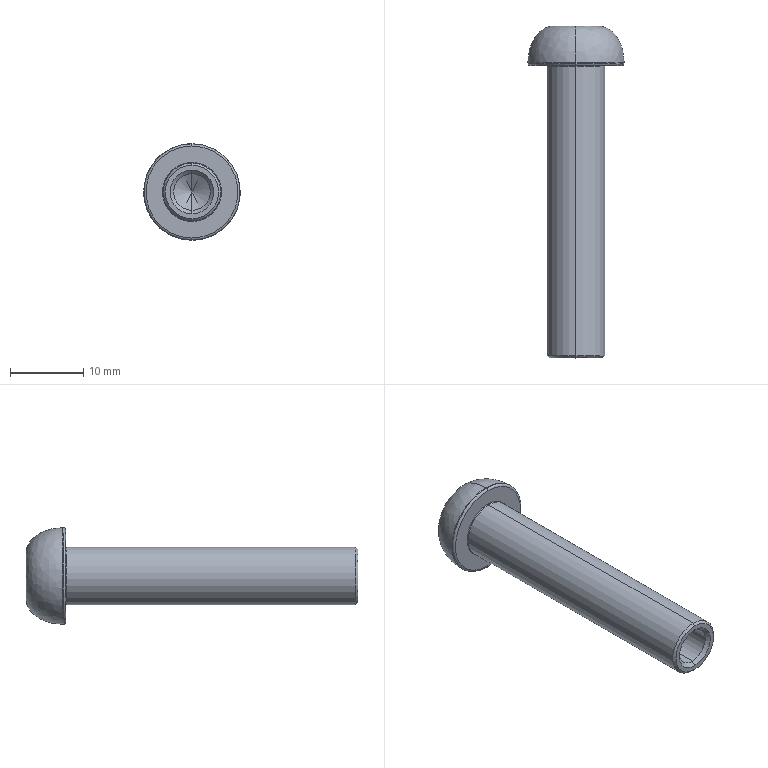Part | SolidWorks | features BaseBody 1 | 1 solid | 38 faces | box 13.2 x 45.4 x 13.2 mm | volume 2174 mm3 | plane 20 | cone 6 | cylinder 6 | torus 4 | spline 2 | commonest cylinder face diameters 5 x2 7.9 x2 13.2 x2
STEP:
#1=CARTESIAN_POINT('',(376.812,-23.5,148.8));
#2=VERTEX_POINT('',#1);
#3=CARTESIAN_POINT('',(376.812,-23.5,153.8));
#4=VERTEX_POINT('',#3);
#5=CARTESIAN_POINT('',(376.812,-23.5,151.3));
#6=DIRECTION('',(0.,1.,0.));
#7=DIRECTION('',(0.,0.,-1.));
#8=AXIS2_PLACEMENT_3D('',#5,#6,#7);
#9=CIRCLE('',#8,2.5);
#10=EDGE_CURVE('',#2,#4,#9,.T.);
#11=ORIENTED_EDGE('',*,*,#10,.T.);
#12=CARTESIAN_POINT('',(376.812,-24.,154.3));
#13=VERTEX_POINT('',#12);
#14=CARTESIAN_POINT('',(376.812,-23.75,154.05));
#15=DIRECTION('',(0.,-0.7071,0.7071));
#16=VECTOR('',#15,1000.);
#17=LINE('',#14,#16);
#18=EDGE_CURVE('',#4,#13,#17,.T.);
#19=ORIENTED_EDGE('',*,*,#18,.T.);
#20=CARTESIAN_POINT('',(376.812,-24.,148.3));
#21=VERTEX_POINT('',#20);
#22=CARTESIAN_POINT('',(376.812,-24.,151.3));
#23=DIRECTION('',(0.,1.,0.));
#24=DIRECTION('',(0.,0.,-1.));
#25=AXIS2_PLACEMENT_3D('',#22,#23,#24);
#26=CIRCLE('',#25,3.);
#27=EDGE_CURVE('',#21,#13,#26,.T.);
#28=ORIENTED_EDGE('',*,*,#27,.F.);
#29=CARTESIAN_POINT('',(376.812,-23.75,148.55));
#30=DIRECTION('',(0.,-0.7071,-0.7071));
#31=VECTOR('',#30,1000.);
#32=LINE('',#29,#31);
#33=EDGE_CURVE('',#2,#21,#32,.T.);
#34=ORIENTED_EDGE('',*,*,#33,.F.);
#35=EDGE_LOOP('',(#11,#19,#28,#34));
#36=FACE_OUTER_BOUND('',#35,.T.);
#37=CARTESIAN_POINT('',(376.812,-23.75,151.3));
#38=DIRECTION('',(0.,-1.,0.));
#39=DIRECTION('',(0.,0.,-1.));
#40=AXIS2_PLACEMENT_3D('',#37,#38,#39);
#41=CONICAL_SURFACE('',#40,2.75,0.7854);
#42=ADVANCED_FACE('',(#36),#41,.F.);
#43=CARTESIAN_POINT('',(376.812,-9.,153.8));
#44=VERTEX_POINT('',#43);
#45=CARTESIAN_POINT('',(376.812,-9.,148.8));
#46=VERTEX_POINT('',#45);
#47=CARTESIAN_POINT('',(376.812,-9.,151.3));
#48=DIRECTION('',(0.,-1.,0.));
#49=DIRECTION('',(0.,0.,1.));
#50=AXIS2_PLACEMENT_3D('',#47,#48,#49);
#51=CIRCLE('',#50,2.5);
#52=EDGE_CURVE('',#44,#46,#51,.T.);
#53=ORIENTED_EDGE('',*,*,#52,.F.);
#54=CARTESIAN_POINT('',(376.812,-9.,153.8));
#55=DIRECTION('',(0.,-1.,0.));
#56=VECTOR('',#55,1000.);
#57=LINE('',#54,#56);
#58=EDGE_CURVE('',#44,#4,#57,.T.);
#59=ORIENTED_EDGE('',*,*,#58,.T.);
#60=ORIENTED_EDGE('',*,*,#10,.F.);
#61=CARTESIAN_POINT('',(376.812,-9.,148.8));
#62=DIRECTION('',(0.,-1.,0.));
#63=VECTOR('',#62,1000.);
#64=LINE('',#61,#63);
#65=EDGE_CURVE('',#46,#2,#64,.T.);
#66=ORIENTED_EDGE('',*,*,#65,.F.);
#67=EDGE_LOOP('',(#53,#59,#60,#66));
#68=FACE_OUTER_BOUND('',#67,.T.);
#69=CARTESIAN_POINT('',(376.812,-9.,151.3));
#70=DIRECTION('',(0.,-1.,0.));
#71=DIRECTION('',(0.,0.,-1.));
#72=AXIS2_PLACEMENT_3D('',#69,#70,#71);
#73=CYLINDRICAL_SURFACE('',#72,2.5);
#74=ADVANCED_FACE('',(#68),#73,.F.);
#75=CARTESIAN_POINT('',(376.812,-7.557,151.3));
#76=VERTEX_POINT('',#75);
#77=CARTESIAN_POINT('',(376.812,-8.293,150.024));
#78=DIRECTION('',(0.,-0.5,-0.866));
#79=VECTOR('',#78,1000.);
#80=LINE('',#77,#79);
#81=EDGE_CURVE('',#76,#46,#80,.T.);
#82=ORIENTED_EDGE('',*,*,#81,.F.);
#83=CARTESIAN_POINT('',(376.812,-8.293,152.576));
#84=DIRECTION('',(0.,-0.5,0.866));
#85=VECTOR('',#84,1000.);
#86=LINE('',#83,#85);
#87=EDGE_CURVE('',#76,#44,#86,.T.);
#88=ORIENTED_EDGE('',*,*,#87,.T.);
#89=ORIENTED_EDGE('',*,*,#52,.T.);
#90=EDGE_LOOP('',(#82,#88,#89));
#91=FACE_OUTER_BOUND('',#90,.T.);
#92=CARTESIAN_POINT('',(376.812,-8.293,151.3));
#93=DIRECTION('',(0.,-1.,0.));
#94=DIRECTION('',(0.,0.,-1.));
#95=AXIS2_PLACEMENT_3D('',#92,#93,#94);
#96=CONICAL_SURFACE('',#95,1.276,1.047);
#97=ADVANCED_FACE('',(#91),#96,.F.);
#98=CARTESIAN_POINT('',(376.812,16.,147.25));
#99=VERTEX_POINT('',#98);
#100=CARTESIAN_POINT('',(376.812,16.,155.35));
#101=VERTEX_POINT('',#100);
#102=CARTESIAN_POINT('',(376.812,16.,151.3));
#103=DIRECTION('',(0.,1.,0.));
#104=DIRECTION('',(0.,0.,-1.));
#105=AXIS2_PLACEMENT_3D('',#102,#103,#104);
#106=CIRCLE('',#105,4.05);
#107=EDGE_CURVE('',#99,#101,#106,.T.);
#108=ORIENTED_EDGE('',*,*,#107,.F.);
#109=CARTESIAN_POINT('',(376.812,15.9,147.35));
#110=VERTEX_POINT('',#109);
#111=CARTESIAN_POINT('',(376.812,15.9,147.25));
#112=DIRECTION('',(1.,0.,0.));
#113=DIRECTION('',(0.,0.,-1.));
#114=AXIS2_PLACEMENT_3D('',#111,#112,#113);
#115=CIRCLE('',#114,0.1);
#116=EDGE_CURVE('',#99,#110,#115,.T.);
#117=ORIENTED_EDGE('',*,*,#116,.T.);
#118=CARTESIAN_POINT('',(376.812,15.9,155.25));
#119=VERTEX_POINT('',#118);
#120=CARTESIAN_POINT('',(376.812,15.9,151.3));
#121=DIRECTION('',(0.,1.,0.));
#122=DIRECTION('',(0.,0.,-1.));
#123=AXIS2_PLACEMENT_3D('',#120,#121,#122);
#124=CIRCLE('',#123,3.95);
#125=EDGE_CURVE('',#110,#119,#124,.T.);
#126=ORIENTED_EDGE('',*,*,#125,.T.);
#127=CARTESIAN_POINT('',(376.812,15.9,155.35));
#128=DIRECTION('',(-1.,0.,0.));
#129=DIRECTION('',(0.,0.,1.));
#130=AXIS2_PLACEMENT_3D('',#127,#128,#129);
#131=CIRCLE('',#130,0.1);
#132=EDGE_CURVE('',#101,#119,#131,.T.);
#133=ORIENTED_EDGE('',*,*,#132,.F.);
#134=EDGE_LOOP('',(#108,#117,#126,#133));
#135=FACE_OUTER_BOUND('',#134,.T.);
#136=CARTESIAN_POINT('',(376.812,15.9,151.3));
#137=DIRECTION('',(0.,1.,0.));
#138=DIRECTION('',(0.,0.,1.));
#139=AXIS2_PLACEMENT_3D('',#136,#137,#138);
#140=TOROIDAL_SURFACE('',#139,4.05,0.1);
#141=ADVANCED_FACE('',(#135),#140,.F.);
#142=CARTESIAN_POINT('',(376.812,16.4,157.9));
#143=VERTEX_POINT('',#142);
#144=CARTESIAN_POINT('',(376.812,16.4,144.7));
#145=VERTEX_POINT('',#144);
#146=CARTESIAN_POINT('',(376.812,16.4,157.9));
#147=CARTESIAN_POINT('',(390.012,16.4,157.9));
#148=CARTESIAN_POINT('',(390.012,16.4,144.7));
#149=CARTESIAN_POINT('',(376.812,16.4,144.7));
#150=(BOUNDED_CURVE()B_SPLINE_CURVE(3,(#146,#147,#148,#149),.UNSPECIFIED.,.F.,.F.)B_SPLINE_CURVE_WITH_KNOTS((4,4),(0.,1.),.UNSPECIFIED.)CURVE()GEOMETRIC_REPRESENTATION_ITEM()RATIONAL_B_SPLINE_CURVE((1.,0.3333,0.3333,1.))REPRESENTATION_ITEM(''));
#151=EDGE_CURVE('',#143,#145,#150,.T.);
#152=ORIENTED_EDGE('',*,*,#151,.F.);
#153=CARTESIAN_POINT('',(376.812,16.3,157.9));
#154=VERTEX_POINT('',#153);
#155=CARTESIAN_POINT('',(376.812,21.4,157.9));
#156=DIRECTION('',(0.,-1.,0.));
#157=VECTOR('',#156,1000.);
#158=LINE('',#155,#157);
#159=EDGE_CURVE('',#143,#154,#158,.T.);
#160=ORIENTED_EDGE('',*,*,#159,.T.);
#161=CARTESIAN_POINT('',(376.812,16.3,144.7));
#162=VERTEX_POINT('',#161);
#163=CARTESIAN_POINT('',(376.812,16.3,151.3));
#164=DIRECTION('',(0.,-1.,0.));
#165=DIRECTION('',(0.,0.,-1.));
#166=AXIS2_PLACEMENT_3D('',#163,#164,#165);
#167=CIRCLE('',#166,6.6);
#168=EDGE_CURVE('',#162,#154,#167,.T.);
#169=ORIENTED_EDGE('',*,*,#168,.F.);
#170=CARTESIAN_POINT('',(376.812,21.4,144.7));
#171=DIRECTION('',(0.,-1.,0.));
#172=VECTOR('',#171,1000.);
#173=LINE('',#170,#172);
#174=EDGE_CURVE('',#145,#162,#173,.T.);
#175=ORIENTED_EDGE('',*,*,#174,.F.);
#176=EDGE_LOOP('',(#152,#160,#169,#175));
#177=FACE_OUTER_BOUND('',#176,.T.);
#178=CARTESIAN_POINT('',(376.812,21.4,151.3));
#179=DIRECTION('',(0.,-1.,0.));
#180=DIRECTION('',(0.,0.,-1.));
#181=AXIS2_PLACEMENT_3D('',#178,#179,#180);
#182=CYLINDRICAL_SURFACE('',#181,6.6);
#183=ADVANCED_FACE('',(#177),#182,.T.);
#184=CARTESIAN_POINT('',(376.812,16.,145.));
#185=VERTEX_POINT('',#184);
#186=CARTESIAN_POINT('',(376.812,16.,157.6));
#187=VERTEX_POINT('',#186);
#188=CARTESIAN_POINT('',(376.812,16.,151.3));
#189=DIRECTION('',(0.,-1.,0.));
#190=DIRECTION('',(0.,0.,1.));
#191=AXIS2_PLACEMENT_3D('',#188,#189,#190);
#192=CIRCLE('',#191,6.3);
#193=EDGE_CURVE('',#185,#187,#192,.T.);
#194=ORIENTED_EDGE('',*,*,#193,.F.);
#195=CARTESIAN_POINT('',(376.812,16.3,145.));
#196=DIRECTION('',(1.,0.,0.));
#197=DIRECTION('',(0.,0.,-1.));
#198=AXIS2_PLACEMENT_3D('',#195,#196,#197);
#199=CIRCLE('',#198,0.3);
#200=EDGE_CURVE('',#185,#162,#199,.T.);
#201=ORIENTED_EDGE('',*,*,#200,.T.);
#202=ORIENTED_EDGE('',*,*,#168,.T.);
#203=CARTESIAN_POINT('',(376.812,16.3,157.6));
#204=DIRECTION('',(-1.,0.,0.));
#205=DIRECTION('',(0.,0.,1.));
#206=AXIS2_PLACEMENT_3D('',#203,#204,#205);
#207=CIRCLE('',#206,0.3);
#208=EDGE_CURVE('',#187,#154,#207,.T.);
#209=ORIENTED_EDGE('',*,*,#208,.F.);
#210=EDGE_LOOP('',(#194,#201,#202,#209));
#211=FACE_OUTER_BOUND('',#210,.T.);
#212=CARTESIAN_POINT('',(376.812,16.3,151.3));
#213=DIRECTION('',(0.,1.,0.));
#214=DIRECTION('',(0.,0.,1.));
#215=AXIS2_PLACEMENT_3D('',#212,#213,#214);
#216=TOROIDAL_SURFACE('',#215,6.3,0.3);
#217=ADVANCED_FACE('',(#211),#216,.T.);
#218=CARTESIAN_POINT('',(376.812,-23.7,147.35));
#219=VERTEX_POINT('',#218);
#220=CARTESIAN_POINT('',(376.812,-23.7,155.25));
#221=VERTEX_POINT('',#220);
#222=CARTESIAN_POINT('',(376.812,-23.7,151.3));
#223=DIRECTION('',(0.,-1.,0.));
#224=DIRECTION('',(0.,0.,-1.));
#225=AXIS2_PLACEMENT_3D('',#222,#223,#224);
#226=CIRCLE('',#225,3.95);
#227=EDGE_CURVE('',#219,#221,#226,.T.);
#228=ORIENTED_EDGE('',*,*,#227,.F.);
#229=CARTESIAN_POINT('',(376.812,-24.,147.35));
#230=DIRECTION('',(0.,1.,0.));
#231=VECTOR('',#230,1000.);
#232=LINE('',#229,#231);
#233=EDGE_CURVE('',#219,#110,#232,.T.);
#234=ORIENTED_EDGE('',*,*,#233,.T.);
#235=CARTESIAN_POINT('',(376.812,15.9,151.3));
#236=DIRECTION('',(0.,1.,0.));
#237=DIRECTION('',(0.,0.,-1.));
#238=AXIS2_PLACEMENT_3D('',#235,#236,#237);
#239=CIRCLE('',#238,3.95);
#240=EDGE_CURVE('',#119,#110,#239,.T.);
#241=ORIENTED_EDGE('',*,*,#240,.F.);
#242=CARTESIAN_POINT('',(376.812,-24.,155.25));
#243=DIRECTION('',(0.,1.,0.));
#244=VECTOR('',#243,1000.);
#245=LINE('',#242,#244);
#246=EDGE_CURVE('',#221,#119,#245,.T.);
#247=ORIENTED_EDGE('',*,*,#246,.F.);
#248=EDGE_LOOP('',(#228,#234,#241,#247));
#249=FACE_OUTER_BOUND('',#248,.T.);
#250=CARTESIAN_POINT('',(376.812,-24.,151.3));
#251=DIRECTION('',(0.,1.,0.));
#252=DIRECTION('',(0.,0.,1.));
#253=AXIS2_PLACEMENT_3D('',#250,#251,#252);
#254=CYLINDRICAL_SURFACE('',#253,3.95);
#255=ADVANCED_FACE('',(#249),#254,.T.);
#256=CARTESIAN_POINT('',(376.812,-24.,147.65));
#257=VERTEX_POINT('',#256);
#258=CARTESIAN_POINT('',(376.812,-24.,154.95));
#259=VERTEX_POINT('',#258);
#260=CARTESIAN_POINT('',(376.812,-24.,151.3));
#261=DIRECTION('',(0.,-1.,0.));
#262=DIRECTION('',(0.,0.,-1.));
#263=AXIS2_PLACEMENT_3D('',#260,#261,#262);
#264=CIRCLE('',#263,3.65);
#265=EDGE_CURVE('',#257,#259,#264,.T.);
#266=ORIENTED_EDGE('',*,*,#265,.F.);
#267=CARTESIAN_POINT('',(376.812,-23.85,147.5));
#268=DIRECTION('',(0.,0.7071,-0.7071));
#269=VECTOR('',#268,1000.);
#270=LINE('',#267,#269);
#271=EDGE_CURVE('',#257,#219,#270,.T.);
#272=ORIENTED_EDGE('',*,*,#271,.T.);
#273=ORIENTED_EDGE('',*,*,#227,.T.);
#274=CARTESIAN_POINT('',(376.812,-23.85,155.1));
#275=DIRECTION('',(0.,0.7071,0.7071));
#276=VECTOR('',#275,1000.);
#277=LINE('',#274,#276);
#278=EDGE_CURVE('',#259,#221,#277,.T.);
#279=ORIENTED_EDGE('',*,*,#278,.F.);
#280=EDGE_LOOP('',(#266,#272,#273,#279));
#281=FACE_OUTER_BOUND('',#280,.T.);
#282=CARTESIAN_POINT('',(376.812,-23.85,151.3));
#283=DIRECTION('',(0.,1.,0.));
#284=DIRECTION('',(0.,0.,1.));
#285=AXIS2_PLACEMENT_3D('',#282,#283,#284);
#286=CONICAL_SURFACE('',#285,3.8,0.7854);
#287=ADVANCED_FACE('',(#281),#286,.T.);
#288=ORIENTED_EDGE('',*,*,#27,.T.);
#289=CARTESIAN_POINT('',(376.812,-24.,151.3));
#290=DIRECTION('',(0.,1.,0.));
#291=DIRECTION('',(0.,0.,-1.));
#292=AXIS2_PLACEMENT_3D('',#289,#290,#291);
#293=CIRCLE('',#292,3.);
#294=EDGE_CURVE('',#13,#21,#293,.T.);
#295=ORIENTED_EDGE('',*,*,#294,.T.);
#296=EDGE_LOOP('',(#288,#295));
#297=FACE_BOUND('',#296,.T.);
#298=CARTESIAN_POINT('',(376.812,-24.,151.3));
#299=DIRECTION('',(0.,-1.,0.));
#300=DIRECTION('',(0.,0.,-1.));
#301=AXIS2_PLACEMENT_3D('',#298,#299,#300);
#302=CIRCLE('',#301,3.65);
#303=EDGE_CURVE('',#259,#257,#302,.T.);
#304=ORIENTED_EDGE('',*,*,#303,.T.);
#305=ORIENTED_EDGE('',*,*,#265,.T.);
#306=EDGE_LOOP('',(#304,#305));
#307=FACE_OUTER_BOUND('',#306,.T.);
#308=CARTESIAN_POINT('',(376.812,-24.,151.3));
#309=DIRECTION('',(0.,-1.,0.));
#310=DIRECTION('',(0.,0.,-1.));
#311=AXIS2_PLACEMENT_3D('',#308,#309,#310);
#312=PLANE('',#311);
#313=ADVANCED_FACE('',(#297,#307),#312,.T.);
#314=ORIENTED_EDGE('',*,*,#271,.F.);
#315=ORIENTED_EDGE('',*,*,#303,.F.);
#316=ORIENTED_EDGE('',*,*,#278,.T.);
#317=CARTESIAN_POINT('',(376.812,-23.7,151.3));
#318=DIRECTION('',(0.,-1.,0.));
#319=DIRECTION('',(0.,0.,-1.));
#320=AXIS2_PLACEMENT_3D('',#317,#318,#319);
#321=CIRCLE('',#320,3.95);
#322=EDGE_CURVE('',#221,#219,#321,.T.);
#323=ORIENTED_EDGE('',*,*,#322,.T.);
#324=EDGE_LOOP('',(#314,#315,#316,#323));
#325=FACE_OUTER_BOUND('',#324,.T.);
#326=CARTESIAN_POINT('',(376.812,-23.85,151.3));
#327=DIRECTION('',(0.,1.,0.));
#328=DIRECTION('',(0.,0.,1.));
#329=AXIS2_PLACEMENT_3D('',#326,#327,#328);
#330=CONICAL_SURFACE('',#329,3.8,0.7854);
#331=ADVANCED_FACE('',(#325),#330,.T.);
#332=ORIENTED_EDGE('',*,*,#233,.F.);
#333=ORIENTED_EDGE('',*,*,#322,.F.);
#334=ORIENTED_EDGE('',*,*,#246,.T.);
#335=ORIENTED_EDGE('',*,*,#125,.F.);
#336=EDGE_LOOP('',(#332,#333,#334,#335));
#337=FACE_OUTER_BOUND('',#336,.T.);
#338=CARTESIAN_POINT('',(376.812,-24.,151.3));
#339=DIRECTION('',(0.,1.,0.));
#340=DIRECTION('',(0.,0.,1.));
#341=AXIS2_PLACEMENT_3D('',#338,#339,#340);
#342=CYLINDRICAL_SURFACE('',#341,3.95);
#343=ADVANCED_FACE('',(#337),#342,.T.);
#344=CARTESIAN_POINT('',(376.812,16.,151.3));
#345=DIRECTION('',(0.,1.,0.));
#346=DIRECTION('',(0.,0.,-1.));
#347=AXIS2_PLACEMENT_3D('',#344,#345,#346);
#348=CIRCLE('',#347,4.05);
#349=EDGE_CURVE('',#101,#99,#348,.T.);
#350=ORIENTED_EDGE('',*,*,#349,.T.);
#351=ORIENTED_EDGE('',*,*,#107,.T.);
#352=EDGE_LOOP('',(#350,#351));
#353=FACE_BOUND('',#352,.T.);
#354=CARTESIAN_POINT('',(376.812,16.,151.3));
#355=DIRECTION('',(0.,-1.,0.));
#356=DIRECTION('',(0.,0.,1.));
#357=AXIS2_PLACEMENT_3D('',#354,#355,#356);
#358=CIRCLE('',#357,6.3);
#359=EDGE_CURVE('',#187,#185,#358,.T.);
#360=ORIENTED_EDGE('',*,*,#359,.T.);
#361=ORIENTED_EDGE('',*,*,#193,.T.);
#362=EDGE_LOOP('',(#360,#361));
#363=FACE_OUTER_BOUND('',#362,.T.);
#364=CARTESIAN_POINT('',(376.812,16.,151.3));
#365=DIRECTION('',(0.,1.,0.));
#366=DIRECTION('',(1.,0.,0.));
#367=AXIS2_PLACEMENT_3D('',#364,#365,#366);
#368=PLANE('',#367);
#369=ADVANCED_FACE('',(#353,#363),#368,.F.);
#370=ORIENTED_EDGE('',*,*,#200,.F.);
#371=ORIENTED_EDGE('',*,*,#359,.F.);
#372=ORIENTED_EDGE('',*,*,#208,.T.);
#373=CARTESIAN_POINT('',(376.812,16.3,151.3));
#374=DIRECTION('',(0.,-1.,0.));
#375=DIRECTION('',(0.,0.,-1.));
#376=AXIS2_PLACEMENT_3D('',#373,#374,#375);
#377=CIRCLE('',#376,6.6);
#378=EDGE_CURVE('',#154,#162,#377,.T.);
#379=ORIENTED_EDGE('',*,*,#378,.T.);
#380=EDGE_LOOP('',(#370,#371,#372,#379));
#381=FACE_OUTER_BOUND('',#380,.T.);
#382=CARTESIAN_POINT('',(376.812,16.3,151.3));
#383=DIRECTION('',(0.,1.,0.));
#384=DIRECTION('',(0.,0.,1.));
#385=AXIS2_PLACEMENT_3D('',#382,#383,#384);
#386=TOROIDAL_SURFACE('',#385,6.3,0.3);
#387=ADVANCED_FACE('',(#381),#386,.T.);
#388=CARTESIAN_POINT('',(376.032,21.4,154.3));
#389=VERTEX_POINT('',#388);
#390=CARTESIAN_POINT('',(376.812,21.4,154.4));
#391=VERTEX_POINT('',#390);
#392=CARTESIAN_POINT('',(376.032,21.4,154.3));
#393=CARTESIAN_POINT('',(376.287,21.4,154.367));
#394=CARTESIAN_POINT('',(376.548,21.4,154.4));
#395=CARTESIAN_POINT('',(376.812,21.4,154.4));
#396=B_SPLINE_CURVE_WITH_KNOTS('',3,(#392,#393,#394,#395),.UNSPECIFIED.,.F.,.F.,(4,4),(0.,1.),.UNSPECIFIED.);
#397=EDGE_CURVE('',#389,#391,#396,.T.);
#398=ORIENTED_EDGE('',*,*,#397,.F.);
#399=CARTESIAN_POINT('',(375.08,21.373,154.3));
#400=VERTEX_POINT('',#399);
#401=CARTESIAN_POINT('',(376.032,21.4,154.3));
#402=CARTESIAN_POINT('',(375.714,21.4,154.3));
#403=CARTESIAN_POINT('',(375.397,21.396,154.3));
#404=CARTESIAN_POINT('',(375.08,21.373,154.3));
#405=B_SPLINE_CURVE_WITH_KNOTS('',3,(#401,#402,#403,#404),.UNSPECIFIED.,.F.,.F.,(4,4),(0.,0.0009518),.UNSPECIFIED.);
#406=EDGE_CURVE('',#389,#400,#405,.T.);
#407=ORIENTED_EDGE('',*,*,#406,.T.);
#408=CARTESIAN_POINT('',(374.605,21.4,153.476));
#409=VERTEX_POINT('',#408);
#410=CARTESIAN_POINT('',(375.08,21.373,154.3));
#411=CARTESIAN_POINT('',(374.922,21.396,154.026));
#412=CARTESIAN_POINT('',(374.763,21.4,153.751));
#413=CARTESIAN_POINT('',(374.605,21.4,153.476));
#414=B_SPLINE_CURVE_WITH_KNOTS('',3,(#410,#411,#412,#413),.UNSPECIFIED.,.F.,.F.,(4,4),(0.,0.0009514),.UNSPECIFIED.);
#415=EDGE_CURVE('',#400,#409,#414,.T.);
#416=ORIENTED_EDGE('',*,*,#415,.T.);
#417=CARTESIAN_POINT('',(373.824,21.4,152.124));
#418=VERTEX_POINT('',#417);
#419=CARTESIAN_POINT('',(374.605,21.4,153.476));
#420=CARTESIAN_POINT('',(374.586,21.4,153.457));
#421=CARTESIAN_POINT('',(374.558,21.4,153.428));
#422=CARTESIAN_POINT('',(374.525,21.4,153.393));
#423=CARTESIAN_POINT('',(374.509,21.4,153.375));
#424=CARTESIAN_POINT('',(374.503,21.4,153.367));
#425=CARTESIAN_POINT('',(374.498,21.4,153.362));
#426=CARTESIAN_POINT('',(374.495,21.4,153.358));
#427=CARTESIAN_POINT('',(374.489,21.4,153.352));
#428=CARTESIAN_POINT('',(374.48,21.4,153.342));
#429=CARTESIAN_POINT('',(374.456,21.4,153.314));
#430=CARTESIAN_POINT('',(374.441,21.4,153.297));
#431=CARTESIAN_POINT('',(374.399,21.4,153.247));
#432=CARTESIAN_POINT('',(374.383,21.4,153.227));
#433=CARTESIAN_POINT('',(374.364,21.4,153.203));
#434=CARTESIAN_POINT('',(374.356,21.4,153.193));
#435=CARTESIAN_POINT('',(374.35,21.4,153.184));
#436=CARTESIAN_POINT('',(374.347,21.4,153.181));
#437=CARTESIAN_POINT('',(374.346,21.4,153.179));
#438=CARTESIAN_POINT('',(374.346,21.4,153.18));
#439=CARTESIAN_POINT('',(374.296,21.4,153.113));
#440=CARTESIAN_POINT('',(374.254,21.4,153.054));
#441=CARTESIAN_POINT('',(374.2,21.4,152.972));
#442=CARTESIAN_POINT('',(374.184,21.4,152.946));
#443=CARTESIAN_POINT('',(374.161,21.4,152.91));
#444=CARTESIAN_POINT('',(374.154,21.4,152.898));
#445=CARTESIAN_POINT('',(374.14,21.4,152.875));
#446=CARTESIAN_POINT('',(374.135,21.4,152.865));
#447=CARTESIAN_POINT('',(374.114,21.4,152.829));
#448=CARTESIAN_POINT('',(374.093,21.4,152.793));
#449=CARTESIAN_POINT('',(374.07,21.4,152.75));
#450=CARTESIAN_POINT('',(374.059,21.4,152.729));
#451=CARTESIAN_POINT('',(374.054,21.4,152.72));
#452=CARTESIAN_POINT('',(374.051,21.4,152.714));
#453=CARTESIAN_POINT('',(374.048,21.4,152.709));
#454=CARTESIAN_POINT('',(374.045,21.4,152.703));
#455=CARTESIAN_POINT('',(374.04,21.4,152.693));
#456=CARTESIAN_POINT('',(374.029,21.4,152.671));
#457=CARTESIAN_POINT('',(374.025,21.4,152.662));
#458=CARTESIAN_POINT('',(374.015,21.4,152.642));
#459=CARTESIAN_POINT('',(374.011,21.4,152.632));
#460=CARTESIAN_POINT('',(373.992,21.4,152.59));
#461=CARTESIAN_POINT('',(373.982,21.4,152.567));
#462=CARTESIAN_POINT('',(373.969,21.4,152.538));
#463=CARTESIAN_POINT('',(373.964,21.4,152.525));
#464=CARTESIAN_POINT('',(373.958,21.4,152.512));
#465=CARTESIAN_POINT('',(373.956,21.4,152.508));
#466=CARTESIAN_POINT('',(373.955,21.4,152.505));
#467=CARTESIAN_POINT('',(373.955,21.4,152.505));
#468=CARTESIAN_POINT('',(373.88,21.4,152.325));
#469=CARTESIAN_POINT('',(373.844,21.4,152.198));
#470=CARTESIAN_POINT('',(373.824,21.4,152.124));
#471=B_SPLINE_CURVE_WITH_KNOTS('',3,(#419,#420,#421,#422,#423,#424,#425,#426,#427,#428,#429,#430,#431,#432,#433,#434,#435,#436,#437,#438,#439,#440,#441,#442,#443,#444,#445,#446,#447,#448,#449,#450,#451,#452,#453,#454,#455,#456,#457,#458,#459,#460,#461,#462,#463,#464,#465,#466,#467,#468,#469,#470),.UNSPECIFIED.,.F.,.F.,(4,1,1,1,2,2,2,2,2,1,1,2,2,2,2,2,2,1,1,1,2,2,2,2,2,2,1,1,2,2,4),(0.,0.0625,0.09375,0.1094,0.1172,0.125,0.1563,0.1875,0.2188,0.2344,0.2422,0.2461,0.25,0.375,0.4375,0.4688,0.5,0.5625,0.5938,0.6094,0.6172,0.625,0.6563,0.6719,0.6875,0.7188,0.7344,0.7422,0.7461,0.75,1.),.UNSPECIFIED.);
#472=EDGE_CURVE('',#409,#418,#471,.T.);
#473=ORIENTED_EDGE('',*,*,#472,.T.);
#474=CARTESIAN_POINT('',(373.348,21.373,151.3));
#475=VERTEX_POINT('',#474);
#476=CARTESIAN_POINT('',(373.824,21.4,152.124));
#477=CARTESIAN_POINT('',(373.665,21.4,151.849));
#478=CARTESIAN_POINT('',(373.507,21.396,151.574));
#479=CARTESIAN_POINT('',(373.348,21.373,151.3));
#480=B_SPLINE_CURVE_WITH_KNOTS('',3,(#476,#477,#478,#479),.UNSPECIFIED.,.F.,.F.,(4,4),(0.,0.000952),.UNSPECIFIED.);
#481=EDGE_CURVE('',#418,#475,#480,.T.);
#482=ORIENTED_EDGE('',*,*,#481,.T.);
#483=CARTESIAN_POINT('',(373.824,21.4,150.476));
#484=VERTEX_POINT('',#483);
#485=CARTESIAN_POINT('',(373.348,21.373,151.3));
#486=CARTESIAN_POINT('',(373.507,21.396,151.026));
#487=CARTESIAN_POINT('',(373.665,21.4,150.751));
#488=CARTESIAN_POINT('',(373.824,21.4,150.476));
#489=B_SPLINE_CURVE_WITH_KNOTS('',3,(#485,#486,#487,#488),.UNSPECIFIED.,.F.,.F.,(4,4),(0.,0.000952),.UNSPECIFIED.);
#490=EDGE_CURVE('',#475,#484,#489,.T.);
#491=ORIENTED_EDGE('',*,*,#490,.T.);
#492=CARTESIAN_POINT('',(374.605,21.4,149.124));
#493=VERTEX_POINT('',#492);
#494=CARTESIAN_POINT('',(373.824,21.4,150.476));
#495=CARTESIAN_POINT('',(373.832,21.4,150.448));
#496=CARTESIAN_POINT('',(373.844,21.4,150.407));
#497=CARTESIAN_POINT('',(373.859,21.4,150.359));
#498=CARTESIAN_POINT('',(373.867,21.4,150.335));
#499=CARTESIAN_POINT('',(373.87,21.4,150.325));
#500=CARTESIAN_POINT('',(373.873,21.4,150.318));
#501=CARTESIAN_POINT('',(373.874,21.4,150.313));
#502=CARTESIAN_POINT('',(373.88,21.4,150.298));
#503=CARTESIAN_POINT('',(373.891,21.4,150.264));
#504=CARTESIAN_POINT('',(373.923,21.4,150.176));
#505=CARTESIAN_POINT('',(373.932,21.4,150.152));
#506=CARTESIAN_POINT('',(373.943,21.4,150.126));
#507=CARTESIAN_POINT('',(373.946,21.4,150.118));
#508=CARTESIAN_POINT('',(373.95,21.4,150.109));
#509=CARTESIAN_POINT('',(373.951,21.4,150.105));
#510=CARTESIAN_POINT('',(373.953,21.4,150.102));
#511=CARTESIAN_POINT('',(373.953,21.4,150.1));
#512=CARTESIAN_POINT('',(373.953,21.4,150.1));
#513=CARTESIAN_POINT('',(373.967,21.4,150.067));
#514=CARTESIAN_POINT('',(373.987,21.4,150.02));
#515=CARTESIAN_POINT('',(374.009,21.4,149.974));
#516=CARTESIAN_POINT('',(374.023,21.4,149.944));
#517=CARTESIAN_POINT('',(374.031,21.4,149.928));
#518=CARTESIAN_POINT('',(374.052,21.4,149.885));
#519=CARTESIAN_POINT('',(374.066,21.4,149.857));
#520=CARTESIAN_POINT('',(374.096,21.4,149.802));
#521=CARTESIAN_POINT('',(374.111,21.4,149.775));
#522=CARTESIAN_POINT('',(374.136,21.4,149.733));
#523=CARTESIAN_POINT('',(374.149,21.4,149.712));
#524=CARTESIAN_POINT('',(374.164,21.4,149.687));
#525=CARTESIAN_POINT('',(374.171,21.4,149.675));
#526=CARTESIAN_POINT('',(374.174,21.4,149.67));
#527=CARTESIAN_POINT('',(374.176,21.4,149.666));
#528=CARTESIAN_POINT('',(374.178,21.4,149.663));
#529=CARTESIAN_POINT('',(374.179,21.4,149.662));
#530=CARTESIAN_POINT('',(374.183,21.4,149.655));
#531=CARTESIAN_POINT('',(374.196,21.4,149.634));
#532=CARTESIAN_POINT('',(374.202,21.4,149.625));
#533=CARTESIAN_POINT('',(374.212,21.4,149.61));
#534=CARTESIAN_POINT('',(374.217,21.4,149.602));
#535=CARTESIAN_POINT('',(374.223,21.4,149.593));
#536=CARTESIAN_POINT('',(374.227,21.4,149.586));
#537=CARTESIAN_POINT('',(374.231,21.4,149.581));
#538=CARTESIAN_POINT('',(374.249,21.4,149.554));
#539=CARTESIAN_POINT('',(374.267,21.4,149.528));
#540=CARTESIAN_POINT('',(374.305,21.4,149.474));
#541=CARTESIAN_POINT('',(374.324,21.4,149.449));
#542=CARTESIAN_POINT('',(374.434,21.4,149.305));
#543=CARTESIAN_POINT('',(374.522,21.4,149.207));
#544=CARTESIAN_POINT('',(374.605,21.4,149.124));
#545=B_SPLINE_CURVE_WITH_KNOTS('',3,(#494,#495,#496,#497,#498,#499,#500,#501,#502,#503,#504,#505,#506,#507,#508,#509,#510,#511,#512,#513,#514,#515,#516,#517,#518,#519,#520,#521,#522,#523,#524,#525,#526,#527,#528,#529,#530,#531,#532,#533,#534,#535,#536,#537,#538,#539,#540,#541,#542,#543,#544),.UNSPECIFIED.,.F.,.F.,(4,1,1,1,2,2,2,2,2,1,2,2,1,2,2,2,2,1,1,1,2,2,2,2,1,2,2,2,2,4),(0.,0.0625,0.09375,0.1094,0.1172,0.125,0.1875,0.2188,0.2344,0.2422,0.2461,0.25,0.3125,0.3438,0.375,0.4375,0.5,0.5312,0.5469,0.5547,0.5586,0.5625,0.5937,0.6094,0.6172,0.6211,0.625,0.6875,0.75,1.),.UNSPECIFIED.);
#546=EDGE_CURVE('',#484,#493,#545,.T.);
#547=ORIENTED_EDGE('',*,*,#546,.T.);
#548=CARTESIAN_POINT('',(375.08,21.373,148.3));
#549=VERTEX_POINT('',#548);
#550=CARTESIAN_POINT('',(374.605,21.4,149.124));
#551=CARTESIAN_POINT('',(374.763,21.4,148.849));
#552=CARTESIAN_POINT('',(374.922,21.396,148.574));
#553=CARTESIAN_POINT('',(375.08,21.373,148.3));
#554=B_SPLINE_CURVE_WITH_KNOTS('',3,(#550,#551,#552,#553),.UNSPECIFIED.,.F.,.F.,(4,4),(0.,0.0009514),.UNSPECIFIED.);
#555=EDGE_CURVE('',#493,#549,#554,.T.);
#556=ORIENTED_EDGE('',*,*,#555,.T.);
#557=CARTESIAN_POINT('',(376.032,21.4,148.3));
#558=VERTEX_POINT('',#557);
#559=CARTESIAN_POINT('',(375.08,21.373,148.3));
#560=CARTESIAN_POINT('',(375.397,21.396,148.3));
#561=CARTESIAN_POINT('',(375.714,21.4,148.3));
#562=CARTESIAN_POINT('',(376.032,21.4,148.3));
#563=B_SPLINE_CURVE_WITH_KNOTS('',3,(#559,#560,#561,#562),.UNSPECIFIED.,.F.,.F.,(4,4),(0.,0.0009518),.UNSPECIFIED.);
#564=EDGE_CURVE('',#549,#558,#563,.T.);
#565=ORIENTED_EDGE('',*,*,#564,.T.);
#566=CARTESIAN_POINT('',(376.812,21.4,148.2));
#567=VERTEX_POINT('',#566);
#568=CARTESIAN_POINT('',(376.812,21.4,148.2));
#569=CARTESIAN_POINT('',(376.548,21.4,148.2));
#570=CARTESIAN_POINT('',(376.287,21.4,148.233));
#571=CARTESIAN_POINT('',(376.032,21.4,148.3));
#572=B_SPLINE_CURVE_WITH_KNOTS('',3,(#568,#569,#570,#571),.UNSPECIFIED.,.F.,.F.,(4,4),(0.,1.),.UNSPECIFIED.);
#573=EDGE_CURVE('',#567,#558,#572,.T.);
#574=ORIENTED_EDGE('',*,*,#573,.F.);
#575=CARTESIAN_POINT('',(376.812,16.4,144.7));
#576=CARTESIAN_POINT('',(376.812,16.981,144.7));
#577=CARTESIAN_POINT('',(376.812,18.257,144.848));
#578=CARTESIAN_POINT('',(376.812,20.059,145.657));
#579=CARTESIAN_POINT('',(376.812,21.195,146.916));
#580=CARTESIAN_POINT('',(376.812,21.4,147.8));
#581=CARTESIAN_POINT('',(376.812,21.4,148.2));
#582=B_SPLINE_CURVE_WITH_KNOTS('',3,(#575,#576,#577,#578,#579,#580,#581),.UNSPECIFIED.,.F.,.F.,(4,1,1,1,4),(0.,0.2463,0.5021,0.7579,1.),.UNSPECIFIED.);
#583=EDGE_CURVE('',#145,#567,#582,.T.);
#584=ORIENTED_EDGE('',*,*,#583,.F.);
#585=CARTESIAN_POINT('',(376.812,16.4,144.7));
#586=CARTESIAN_POINT('',(372.946,16.4,144.7));
#587=CARTESIAN_POINT('',(370.213,16.4,147.434));
#588=CARTESIAN_POINT('',(370.213,16.4,151.3));
#589=CARTESIAN_POINT('',(370.213,16.4,155.166));
#590=CARTESIAN_POINT('',(372.946,16.4,157.9));
#591=CARTESIAN_POINT('',(376.812,16.4,157.9));
#592=(BOUNDED_CURVE()B_SPLINE_CURVE(3,(#585,#586,#587,#588,#589,#590,#591),.UNSPECIFIED.,.F.,.F.)B_SPLINE_CURVE_WITH_KNOTS((4,3,4),(0.,0.5,1.),.UNSPECIFIED.)CURVE()GEOMETRIC_REPRESENTATION_ITEM()RATIONAL_B_SPLINE_CURVE((1.,0.8047,0.8047,1.,0.8047,0.8047,1.))REPRESENTATION_ITEM(''));
#593=EDGE_CURVE('',#145,#143,#592,.T.);
#594=ORIENTED_EDGE('',*,*,#593,.T.);
#595=CARTESIAN_POINT('',(376.812,16.4,157.9));
#596=CARTESIAN_POINT('',(376.812,16.981,157.9));
#597=CARTESIAN_POINT('',(376.812,18.257,157.752));
#598=CARTESIAN_POINT('',(376.812,20.059,156.943));
#599=CARTESIAN_POINT('',(376.812,21.195,155.684));
#600=CARTESIAN_POINT('',(376.812,21.4,154.8));
#601=CARTESIAN_POINT('',(376.812,21.4,154.4));
#602=(BOUNDED_CURVE()B_SPLINE_CURVE(3,(#595,#596,#597,#598,#599,#600,#601),.UNSPECIFIED.,.F.,.F.)B_SPLINE_CURVE_WITH_KNOTS((4,1,1,1,4),(0.,0.2463,0.5021,0.7579,1.),.UNSPECIFIED.)CURVE()GEOMETRIC_REPRESENTATION_ITEM()RATIONAL_B_SPLINE_CURVE((1.,1.,1.,1.,1.,1.,1.))REPRESENTATION_ITEM(''));
#603=EDGE_CURVE('',#143,#391,#602,.T.);
#604=ORIENTED_EDGE('',*,*,#603,.T.);
#605=EDGE_LOOP('',(#398,#407,#416,#473,#482,#491,#547,#556,#565,#574,#584,#594,#604));
#606=FACE_OUTER_BOUND('',#605,.T.);
#607=CARTESIAN_POINT('',(376.812,21.4,154.369));
#608=CARTESIAN_POINT('',(375.014,21.4,154.369));
#609=CARTESIAN_POINT('',(373.743,21.4,153.098));
#610=CARTESIAN_POINT('',(373.743,21.4,151.3));
#611=CARTESIAN_POINT('',(373.743,21.4,149.502));
#612=CARTESIAN_POINT('',(375.014,21.4,148.231));
#613=CARTESIAN_POINT('',(376.812,21.4,148.231));
#614=CARTESIAN_POINT('',(376.812,21.405,154.778));
#615=CARTESIAN_POINT('',(374.775,21.405,154.778));
#616=CARTESIAN_POINT('',(373.335,21.405,153.337));
#617=CARTESIAN_POINT('',(373.335,21.405,151.3));
#618=CARTESIAN_POINT('',(373.335,21.405,149.263));
#619=CARTESIAN_POINT('',(374.775,21.405,147.822));
#620=CARTESIAN_POINT('',(376.812,21.405,147.822));
#621=CARTESIAN_POINT('',(376.812,21.204,155.674));
#622=CARTESIAN_POINT('',(374.25,21.204,155.674));
#623=CARTESIAN_POINT('',(372.438,21.204,153.862));
#624=CARTESIAN_POINT('',(372.438,21.204,151.3));
#625=CARTESIAN_POINT('',(372.438,21.204,148.738));
#626=CARTESIAN_POINT('',(374.25,21.204,146.926));
#627=CARTESIAN_POINT('',(376.812,21.204,146.926));
#628=CARTESIAN_POINT('',(376.812,20.059,156.943));
#629=CARTESIAN_POINT('',(373.507,20.059,156.943));
#630=CARTESIAN_POINT('',(371.169,20.059,154.606));
#631=CARTESIAN_POINT('',(371.169,20.059,151.3));
#632=CARTESIAN_POINT('',(371.169,20.059,147.994));
#633=CARTESIAN_POINT('',(373.507,20.059,145.657));
#634=CARTESIAN_POINT('',(376.812,20.059,145.657));
#635=CARTESIAN_POINT('',(376.812,18.257,157.752));
#636=CARTESIAN_POINT('',(373.033,18.257,157.752));
#637=CARTESIAN_POINT('',(370.36,18.257,155.08));
#638=CARTESIAN_POINT('',(370.36,18.257,151.3));
#639=CARTESIAN_POINT('',(370.36,18.257,147.52));
#640=CARTESIAN_POINT('',(373.033,18.257,144.848));
#641=CARTESIAN_POINT('',(376.812,18.257,144.848));
#642=CARTESIAN_POINT('',(376.812,16.981,157.9));
#643=CARTESIAN_POINT('',(372.946,16.981,157.9));
#644=CARTESIAN_POINT('',(370.213,16.981,155.166));
#645=CARTESIAN_POINT('',(370.213,16.981,151.3));
#646=CARTESIAN_POINT('',(370.213,16.981,147.434));
#647=CARTESIAN_POINT('',(372.946,16.981,144.7));
#648=CARTESIAN_POINT('',(376.812,16.981,144.7));
#649=CARTESIAN_POINT('',(376.812,16.4,157.9));
#650=CARTESIAN_POINT('',(372.946,16.4,157.9));
#651=CARTESIAN_POINT('',(370.213,16.4,155.166));
#652=CARTESIAN_POINT('',(370.213,16.4,151.3));
#653=CARTESIAN_POINT('',(370.213,16.4,147.434));
#654=CARTESIAN_POINT('',(372.946,16.4,144.7));
#655=CARTESIAN_POINT('',(376.812,16.4,144.7));
#656=(BOUNDED_SURFACE()B_SPLINE_SURFACE(3,3,((#607,#608,#609,#610,#611,#612,#613),(#614,#615,#616,#617,#618,#619,#620),(#621,#622,#623,#624,#625,#626,#627),(#628,#629,#630,#631,#632,#633,#634),(#635,#636,#637,#638,#639,#640,#641),(#642,#643,#644,#645,#646,#647,#648),(#649,#650,#651,#652,#653,#654,#655)),.UNSPECIFIED.,.F.,.F.,.F.)B_SPLINE_SURFACE_WITH_KNOTS((4,1,1,1,4),(4,3,4),(0.007322,0.25,0.5,0.75,0.9907),(0.,0.5,1.),.UNSPECIFIED.)GEOMETRIC_REPRESENTATION_ITEM()RATIONAL_B_SPLINE_SURFACE(((1.,0.8047,0.8047,1.,0.8047,0.8047,1.),(1.,0.8047,0.8047,1.,0.8047,0.8047,1.),(1.,0.8047,0.8047,1.,0.8047,0.8047,1.),(1.,0.8047,0.8047,1.,0.8047,0.8047,1.),(1.,0.8047,0.8047,1.,0.8047,0.8047,1.),(1.,0.8047,0.8047,1.,0.8047,0.8047,1.),(1.,0.8047,0.8047,1.,0.8047,0.8047,1.)))REPRESENTATION_ITEM('')SURFACE());
#657=ADVANCED_FACE('',(#606),#656,.F.);
#658=ORIENTED_EDGE('',*,*,#603,.F.);
#659=ORIENTED_EDGE('',*,*,#151,.T.);
#660=ORIENTED_EDGE('',*,*,#583,.T.);
#661=CARTESIAN_POINT('',(377.593,21.4,148.3));
#662=VERTEX_POINT('',#661);
#663=CARTESIAN_POINT('',(377.593,21.4,148.3));
#664=CARTESIAN_POINT('',(377.337,21.4,148.233));
#665=CARTESIAN_POINT('',(377.077,21.4,148.2));
#666=CARTESIAN_POINT('',(376.812,21.4,148.2));
#667=B_SPLINE_CURVE_WITH_KNOTS('',3,(#663,#664,#665,#666),.UNSPECIFIED.,.F.,.F.,(4,4),(0.,1.),.UNSPECIFIED.);
#668=EDGE_CURVE('',#662,#567,#667,.T.);
#669=ORIENTED_EDGE('',*,*,#668,.F.);
#670=CARTESIAN_POINT('',(378.544,21.373,148.3));
#671=VERTEX_POINT('',#670);
#672=CARTESIAN_POINT('',(377.593,21.4,148.3));
#673=CARTESIAN_POINT('',(377.91,21.4,148.3));
#674=CARTESIAN_POINT('',(378.228,21.396,148.3));
#675=CARTESIAN_POINT('',(378.544,21.373,148.3));
#676=B_SPLINE_CURVE_WITH_KNOTS('',3,(#672,#673,#674,#675),.UNSPECIFIED.,.F.,.F.,(4,4),(0.,0.0009518),.UNSPECIFIED.);
#677=EDGE_CURVE('',#662,#671,#676,.T.);
#678=ORIENTED_EDGE('',*,*,#677,.T.);
#679=CARTESIAN_POINT('',(379.02,21.4,149.124));
#680=VERTEX_POINT('',#679);
#681=CARTESIAN_POINT('',(378.544,21.373,148.3));
#682=CARTESIAN_POINT('',(378.703,21.396,148.574));
#683=CARTESIAN_POINT('',(378.861,21.4,148.849));
#684=CARTESIAN_POINT('',(379.02,21.4,149.124));
#685=B_SPLINE_CURVE_WITH_KNOTS('',3,(#681,#682,#683,#684),.UNSPECIFIED.,.F.,.F.,(4,4),(0.,0.0009514),.UNSPECIFIED.);
#686=EDGE_CURVE('',#671,#680,#685,.T.);
#687=ORIENTED_EDGE('',*,*,#686,.T.);
#688=CARTESIAN_POINT('',(379.801,21.4,150.476));
#689=VERTEX_POINT('',#688);
#690=CARTESIAN_POINT('',(379.02,21.4,149.124));
#691=CARTESIAN_POINT('',(379.039,21.4,149.143));
#692=CARTESIAN_POINT('',(379.067,21.4,149.172));
#693=CARTESIAN_POINT('',(379.099,21.4,149.207));
#694=CARTESIAN_POINT('',(379.115,21.4,149.225));
#695=CARTESIAN_POINT('',(379.122,21.4,149.233));
#696=CARTESIAN_POINT('',(379.127,21.4,149.238));
#697=CARTESIAN_POINT('',(379.13,21.4,149.242));
#698=CARTESIAN_POINT('',(379.136,21.4,149.248));
#699=CARTESIAN_POINT('',(379.144,21.4,149.258));
#700=CARTESIAN_POINT('',(379.169,21.4,149.286));
#701=CARTESIAN_POINT('',(379.184,21.4,149.303));
#702=CARTESIAN_POINT('',(379.225,21.4,149.353));
#703=CARTESIAN_POINT('',(379.242,21.4,149.374));
#704=CARTESIAN_POINT('',(379.261,21.4,149.397));
#705=CARTESIAN_POINT('',(379.268,21.4,149.407));
#706=CARTESIAN_POINT('',(379.275,21.4,149.416));
#707=CARTESIAN_POINT('',(379.277,21.4,149.419));
#708=CARTESIAN_POINT('',(379.279,21.4,149.421));
#709=CARTESIAN_POINT('',(379.278,21.4,149.42));
#710=CARTESIAN_POINT('',(379.329,21.4,149.487));
#711=CARTESIAN_POINT('',(379.371,21.4,149.547));
#712=CARTESIAN_POINT('',(379.425,21.4,149.629));
#713=CARTESIAN_POINT('',(379.441,21.4,149.655));
#714=CARTESIAN_POINT('',(379.464,21.4,149.691));
#715=CARTESIAN_POINT('',(379.471,21.4,149.703));
#716=CARTESIAN_POINT('',(379.484,21.4,149.725));
#717=CARTESIAN_POINT('',(379.49,21.4,149.735));
#718=CARTESIAN_POINT('',(379.511,21.4,149.771));
#719=CARTESIAN_POINT('',(379.531,21.4,149.807));
#720=CARTESIAN_POINT('',(379.554,21.4,149.85));
#721=CARTESIAN_POINT('',(379.566,21.4,149.871));
#722=CARTESIAN_POINT('',(379.571,21.4,149.88));
#723=CARTESIAN_POINT('',(379.574,21.4,149.886));
#724=CARTESIAN_POINT('',(379.576,21.4,149.891));
#725=CARTESIAN_POINT('',(379.58,21.4,149.897));
#726=CARTESIAN_POINT('',(379.585,21.4,149.907));
#727=CARTESIAN_POINT('',(379.596,21.4,149.929));
#728=CARTESIAN_POINT('',(379.6,21.4,149.938));
#729=CARTESIAN_POINT('',(379.609,21.4,149.958));
#730=CARTESIAN_POINT('',(379.614,21.4,149.968));
#731=CARTESIAN_POINT('',(379.633,21.4,150.01));
#732=CARTESIAN_POINT('',(379.643,21.4,150.034));
#733=CARTESIAN_POINT('',(379.656,21.4,150.063));
#734=CARTESIAN_POINT('',(379.661,21.4,150.076));
#735=CARTESIAN_POINT('',(379.666,21.4,150.088));
#736=CARTESIAN_POINT('',(379.668,21.4,150.092));
#737=CARTESIAN_POINT('',(379.669,21.4,150.095));
#738=CARTESIAN_POINT('',(379.669,21.4,150.095));
#739=CARTESIAN_POINT('',(379.744,21.4,150.274));
#740=CARTESIAN_POINT('',(379.781,21.4,150.404));
#741=CARTESIAN_POINT('',(379.801,21.4,150.476));
#742=B_SPLINE_CURVE_WITH_KNOTS('',3,(#690,#691,#692,#693,#694,#695,#696,#697,#698,#699,#700,#701,#702,#703,#704,#705,#706,#707,#708,#709,#710,#711,#712,#713,#714,#715,#716,#717,#718,#719,#720,#721,#722,#723,#724,#725,#726,#727,#728,#729,#730,#731,#732,#733,#734,#735,#736,#737,#738,#739,#740,#741),.UNSPECIFIED.,.F.,.F.,(4,1,1,1,2,2,2,2,2,1,1,2,2,2,2,2,2,1,1,1,2,2,2,2,2,2,1,1,2,2,4),(0.,0.0625,0.09375,0.1094,0.1172,0.125,0.1563,0.1875,0.2188,0.2344,0.2422,0.2461,0.25,0.375,0.4375,0.4688,0.5,0.5625,0.5938,0.6094,0.6172,0.625,0.6563,0.6719,0.6875,0.7188,0.7344,0.7422,0.7461,0.75,1.),.UNSPECIFIED.);
#743=EDGE_CURVE('',#680,#689,#742,.T.);
#744=ORIENTED_EDGE('',*,*,#743,.T.);
#745=CARTESIAN_POINT('',(380.276,21.373,151.3));
#746=VERTEX_POINT('',#745);
#747=CARTESIAN_POINT('',(379.801,21.4,150.476));
#748=CARTESIAN_POINT('',(379.959,21.4,150.751));
#749=CARTESIAN_POINT('',(380.118,21.396,151.026));
#750=CARTESIAN_POINT('',(380.276,21.373,151.3));
#751=B_SPLINE_CURVE_WITH_KNOTS('',3,(#747,#748,#749,#750),.UNSPECIFIED.,.F.,.F.,(4,4),(0.,0.000952),.UNSPECIFIED.);
#752=EDGE_CURVE('',#689,#746,#751,.T.);
#753=ORIENTED_EDGE('',*,*,#752,.T.);
#754=CARTESIAN_POINT('',(379.801,21.4,152.124));
#755=VERTEX_POINT('',#754);
#756=CARTESIAN_POINT('',(380.276,21.373,151.3));
#757=CARTESIAN_POINT('',(380.118,21.396,151.574));
#758=CARTESIAN_POINT('',(379.959,21.4,151.849));
#759=CARTESIAN_POINT('',(379.801,21.4,152.124));
#760=B_SPLINE_CURVE_WITH_KNOTS('',3,(#756,#757,#758,#759),.UNSPECIFIED.,.F.,.F.,(4,4),(0.,0.000952),.UNSPECIFIED.);
#761=EDGE_CURVE('',#746,#755,#760,.T.);
#762=ORIENTED_EDGE('',*,*,#761,.T.);
#763=CARTESIAN_POINT('',(379.02,21.4,153.476));
#764=VERTEX_POINT('',#763);
#765=CARTESIAN_POINT('',(379.801,21.4,152.124));
#766=CARTESIAN_POINT('',(379.793,21.4,152.152));
#767=CARTESIAN_POINT('',(379.781,21.4,152.193));
#768=CARTESIAN_POINT('',(379.766,21.4,152.241));
#769=CARTESIAN_POINT('',(379.758,21.4,152.265));
#770=CARTESIAN_POINT('',(379.754,21.4,152.275));
#771=CARTESIAN_POINT('',(379.752,21.4,152.282));
#772=CARTESIAN_POINT('',(379.75,21.4,152.287));
#773=CARTESIAN_POINT('',(379.745,21.4,152.302));
#774=CARTESIAN_POINT('',(379.734,21.4,152.336));
#775=CARTESIAN_POINT('',(379.702,21.4,152.424));
#776=CARTESIAN_POINT('',(379.693,21.4,152.447));
#777=CARTESIAN_POINT('',(379.682,21.4,152.474));
#778=CARTESIAN_POINT('',(379.677,21.4,152.485));
#779=CARTESIAN_POINT('',(379.674,21.4,152.495));
#780=CARTESIAN_POINT('',(379.672,21.4,152.498));
#781=CARTESIAN_POINT('',(379.671,21.4,152.5));
#782=CARTESIAN_POINT('',(379.671,21.4,152.5));
#783=CARTESIAN_POINT('',(379.658,21.4,152.533));
#784=CARTESIAN_POINT('',(379.637,21.4,152.58));
#785=CARTESIAN_POINT('',(379.616,21.4,152.626));
#786=CARTESIAN_POINT('',(379.602,21.4,152.656));
#787=CARTESIAN_POINT('',(379.594,21.4,152.672));
#788=CARTESIAN_POINT('',(379.573,21.4,152.715));
#789=CARTESIAN_POINT('',(379.559,21.4,152.743));
#790=CARTESIAN_POINT('',(379.529,21.4,152.798));
#791=CARTESIAN_POINT('',(379.514,21.4,152.825));
#792=CARTESIAN_POINT('',(379.489,21.4,152.867));
#793=CARTESIAN_POINT('',(379.476,21.4,152.888));
#794=CARTESIAN_POINT('',(379.461,21.4,152.913));
#795=CARTESIAN_POINT('',(379.454,21.4,152.925));
#796=CARTESIAN_POINT('',(379.451,21.4,152.93));
#797=CARTESIAN_POINT('',(379.448,21.4,152.934));
#798=CARTESIAN_POINT('',(379.446,21.4,152.937));
#799=CARTESIAN_POINT('',(379.446,21.4,152.938));
#800=CARTESIAN_POINT('',(379.441,21.4,152.945));
#801=CARTESIAN_POINT('',(379.428,21.4,152.966));
#802=CARTESIAN_POINT('',(379.423,21.4,152.975));
#803=CARTESIAN_POINT('',(379.413,21.4,152.99));
#804=CARTESIAN_POINT('',(379.407,21.4,152.998));
#805=CARTESIAN_POINT('',(379.401,21.4,153.007));
#806=CARTESIAN_POINT('',(379.397,21.4,153.014));
#807=CARTESIAN_POINT('',(379.394,21.4,153.019));
#808=CARTESIAN_POINT('',(379.376,21.4,153.046));
#809=CARTESIAN_POINT('',(379.358,21.4,153.072));
#810=CARTESIAN_POINT('',(379.319,21.4,153.126));
#811=CARTESIAN_POINT('',(379.301,21.4,153.151));
#812=CARTESIAN_POINT('',(379.19,21.4,153.296));
#813=CARTESIAN_POINT('',(379.102,21.4,153.394));
#814=CARTESIAN_POINT('',(379.02,21.4,153.476));
#815=B_SPLINE_CURVE_WITH_KNOTS('',3,(#765,#766,#767,#768,#769,#770,#771,#772,#773,#774,#775,#776,#777,#778,#779,#780,#781,#782,#783,#784,#785,#786,#787,#788,#789,#790,#791,#792,#793,#794,#795,#796,#797,#798,#799,#800,#801,#802,#803,#804,#805,#806,#807,#808,#809,#810,#811,#812,#813,#814),.UNSPECIFIED.,.F.,.F.,(4,1,1,1,2,2,2,2,1,1,2,2,1,2,2,2,2,1,1,1,2,2,2,2,1,2,2,2,2,4),(0.,0.0625,0.09375,0.1094,0.1172,0.125,0.1875,0.2188,0.2344,0.2422,0.2461,0.25,0.3125,0.3438,0.375,0.4375,0.5,0.5313,0.5469,0.5547,0.5586,0.5625,0.5938,0.6094,0.6172,0.6211,0.625,0.6875,0.75,1.),.UNSPECIFIED.);
#816=EDGE_CURVE('',#755,#764,#815,.T.);
#817=ORIENTED_EDGE('',*,*,#816,.T.);
#818=CARTESIAN_POINT('',(378.544,21.373,154.3));
#819=VERTEX_POINT('',#818);
#820=CARTESIAN_POINT('',(379.02,21.4,153.476));
#821=CARTESIAN_POINT('',(378.861,21.4,153.751));
#822=CARTESIAN_POINT('',(378.703,21.396,154.026));
#823=CARTESIAN_POINT('',(378.544,21.373,154.3));
#824=B_SPLINE_CURVE_WITH_KNOTS('',3,(#820,#821,#822,#823),.UNSPECIFIED.,.F.,.F.,(4,4),(0.,0.0009514),.UNSPECIFIED.);
#825=EDGE_CURVE('',#764,#819,#824,.T.);
#826=ORIENTED_EDGE('',*,*,#825,.T.);
#827=CARTESIAN_POINT('',(377.593,21.4,154.3));
#828=VERTEX_POINT('',#827);
#829=CARTESIAN_POINT('',(378.544,21.373,154.3));
#830=CARTESIAN_POINT('',(378.228,21.396,154.3));
#831=CARTESIAN_POINT('',(377.91,21.4,154.3));
#832=CARTESIAN_POINT('',(377.593,21.4,154.3));
#833=B_SPLINE_CURVE_WITH_KNOTS('',3,(#829,#830,#831,#832),.UNSPECIFIED.,.F.,.F.,(4,4),(0.,0.0009518),.UNSPECIFIED.);
#834=EDGE_CURVE('',#819,#828,#833,.T.);
#835=ORIENTED_EDGE('',*,*,#834,.T.);
#836=CARTESIAN_POINT('',(376.812,21.4,154.4));
#837=CARTESIAN_POINT('',(377.077,21.4,154.4));
#838=CARTESIAN_POINT('',(377.337,21.4,154.367));
#839=CARTESIAN_POINT('',(377.593,21.4,154.3));
#840=B_SPLINE_CURVE_WITH_KNOTS('',3,(#836,#837,#838,#839),.UNSPECIFIED.,.F.,.F.,(4,4),(0.,1.),.UNSPECIFIED.);
#841=EDGE_CURVE('',#391,#828,#840,.T.);
#842=ORIENTED_EDGE('',*,*,#841,.F.);
#843=EDGE_LOOP('',(#658,#659,#660,#669,#678,#687,#744,#753,#762,#817,#826,#835,#842));
#844=FACE_OUTER_BOUND('',#843,.T.);
#845=CARTESIAN_POINT('',(376.812,21.4,148.231));
#846=CARTESIAN_POINT('',(382.951,21.4,148.231));
#847=CARTESIAN_POINT('',(382.951,21.4,154.369));
#848=CARTESIAN_POINT('',(376.812,21.4,154.369));
#849=CARTESIAN_POINT('',(376.812,21.405,147.822));
#850=CARTESIAN_POINT('',(383.768,21.405,147.822));
#851=CARTESIAN_POINT('',(383.768,21.405,154.778));
#852=CARTESIAN_POINT('',(376.812,21.405,154.778));
#853=CARTESIAN_POINT('',(376.812,21.204,146.926));
#854=CARTESIAN_POINT('',(385.56,21.204,146.926));
#855=CARTESIAN_POINT('',(385.56,21.204,155.674));
#856=CARTESIAN_POINT('',(376.812,21.204,155.674));
#857=CARTESIAN_POINT('',(376.812,20.059,145.657));
#858=CARTESIAN_POINT('',(388.099,20.059,145.657));
#859=CARTESIAN_POINT('',(388.099,20.059,156.943));
#860=CARTESIAN_POINT('',(376.812,20.059,156.943));
#861=CARTESIAN_POINT('',(376.812,18.257,144.848));
#862=CARTESIAN_POINT('',(389.717,18.257,144.848));
#863=CARTESIAN_POINT('',(389.717,18.257,157.752));
#864=CARTESIAN_POINT('',(376.812,18.257,157.752));
#865=CARTESIAN_POINT('',(376.812,16.981,144.7));
#866=CARTESIAN_POINT('',(390.012,16.981,144.7));
#867=CARTESIAN_POINT('',(390.012,16.981,157.9));
#868=CARTESIAN_POINT('',(376.812,16.981,157.9));
#869=CARTESIAN_POINT('',(376.812,16.4,144.7));
#870=CARTESIAN_POINT('',(390.012,16.4,144.7));
#871=CARTESIAN_POINT('',(390.012,16.4,157.9));
#872=CARTESIAN_POINT('',(376.812,16.4,157.9));
#873=(BOUNDED_SURFACE()B_SPLINE_SURFACE(3,3,((#845,#846,#847,#848),(#849,#850,#851,#852),(#853,#854,#855,#856),(#857,#858,#859,#860),(#861,#862,#863,#864),(#865,#866,#867,#868),(#869,#870,#871,#872)),.UNSPECIFIED.,.F.,.F.,.T.)B_SPLINE_SURFACE_WITH_KNOTS((4,1,1,1,4),(4,4),(0.007322,0.25,0.5,0.75,0.9907),(0.,1.),.UNSPECIFIED.)GEOMETRIC_REPRESENTATION_ITEM()RATIONAL_B_SPLINE_SURFACE(((1.,0.3333,0.3333,1.),(1.,0.3333,0.3333,1.),(1.,0.3333,0.3333,1.),(1.,0.3333,0.3333,1.),(1.,0.3333,0.3333,1.),(1.,0.3333,0.3333,1.),(1.,0.3333,0.3333,1.)))REPRESENTATION_ITEM('')SURFACE());
#874=ADVANCED_FACE('',(#844),#873,.F.);
#875=ORIENTED_EDGE('',*,*,#397,.T.);
#876=ORIENTED_EDGE('',*,*,#841,.T.);
#877=CARTESIAN_POINT('',(377.593,21.4,154.3));
#878=DIRECTION('',(-1.,0.,0.));
#879=VECTOR('',#878,1000.);
#880=LINE('',#877,#879);
#881=EDGE_CURVE('',#828,#389,#880,.T.);
#882=ORIENTED_EDGE('',*,*,#881,.T.);
#883=EDGE_LOOP('',(#875,#876,#882));
#884=FACE_OUTER_BOUND('',#883,.T.);
#885=CARTESIAN_POINT('',(376.812,21.4,151.3));
#886=DIRECTION('',(0.,1.,0.));
#887=DIRECTION('',(1.,0.,0.));
#888=AXIS2_PLACEMENT_3D('',#885,#886,#887);
#889=PLANE('',#888);
#890=ADVANCED_FACE('',(#884),#889,.T.);
#891=ORIENTED_EDGE('',*,*,#406,.F.);
#892=ORIENTED_EDGE('',*,*,#881,.F.);
#893=ORIENTED_EDGE('',*,*,#834,.F.);
#894=CARTESIAN_POINT('',(378.544,19.4,154.3));
#895=VERTEX_POINT('',#894);
#896=CARTESIAN_POINT('',(378.544,19.4,154.3));
#897=DIRECTION('',(0.,-1.,0.));
#898=VECTOR('',#897,1000.);
#899=LINE('',#896,#898);
#900=EDGE_CURVE('',#819,#895,#899,.T.);
#901=ORIENTED_EDGE('',*,*,#900,.T.);
#902=CARTESIAN_POINT('',(375.08,19.4,154.3));
#903=VERTEX_POINT('',#902);
#904=CARTESIAN_POINT('',(378.544,19.4,154.3));
#905=DIRECTION('',(-1.,0.,0.));
#906=VECTOR('',#905,1000.);
#907=LINE('',#904,#906);
#908=EDGE_CURVE('',#895,#903,#907,.T.);
#909=ORIENTED_EDGE('',*,*,#908,.T.);
#910=CARTESIAN_POINT('',(375.08,19.4,154.3));
#911=DIRECTION('',(0.,-1.,0.));
#912=VECTOR('',#911,1000.);
#913=LINE('',#910,#912);
#914=EDGE_CURVE('',#400,#903,#913,.T.);
#915=ORIENTED_EDGE('',*,*,#914,.F.);
#916=EDGE_LOOP('',(#891,#892,#893,#901,#909,#915));
#917=FACE_OUTER_BOUND('',#916,.T.);
#918=CARTESIAN_POINT('',(375.08,19.4,154.3));
#919=DIRECTION('',(0.,0.,1.));
#920=DIRECTION('',(1.,0.,0.));
#921=AXIS2_PLACEMENT_3D('',#918,#919,#920);
#922=PLANE('',#921);
#923=ADVANCED_FACE('',(#917),#922,.F.);
#924=ORIENTED_EDGE('',*,*,#481,.F.);
#925=CARTESIAN_POINT('',(374.605,21.4,153.476));
#926=DIRECTION('',(-0.5,0.,-0.866));
#927=VECTOR('',#926,1000.);
#928=LINE('',#925,#927);
#929=EDGE_CURVE('',#409,#418,#928,.T.);
#930=ORIENTED_EDGE('',*,*,#929,.F.);
#931=ORIENTED_EDGE('',*,*,#415,.F.);
#932=ORIENTED_EDGE('',*,*,#914,.T.);
#933=CARTESIAN_POINT('',(373.348,19.4,151.3));
#934=VERTEX_POINT('',#933);
#935=CARTESIAN_POINT('',(373.348,19.4,151.3));
#936=DIRECTION('',(0.5,0.,0.866));
#937=VECTOR('',#936,1000.);
#938=LINE('',#935,#937);
#939=EDGE_CURVE('',#934,#903,#938,.T.);
#940=ORIENTED_EDGE('',*,*,#939,.F.);
#941=CARTESIAN_POINT('',(373.348,19.4,151.3));
#942=DIRECTION('',(0.,-1.,0.));
#943=VECTOR('',#942,1000.);
#944=LINE('',#941,#943);
#945=EDGE_CURVE('',#475,#934,#944,.T.);
#946=ORIENTED_EDGE('',*,*,#945,.F.);
#947=EDGE_LOOP('',(#924,#930,#931,#932,#940,#946));
#948=FACE_OUTER_BOUND('',#947,.T.);
#949=CARTESIAN_POINT('',(373.348,19.4,151.3));
#950=DIRECTION('',(-0.866,0.,0.5));
#951=DIRECTION('',(0.,1.,0.));
#952=AXIS2_PLACEMENT_3D('',#949,#950,#951);
#953=PLANE('',#952);
#954=ADVANCED_FACE('',(#948),#953,.F.);
#955=ORIENTED_EDGE('',*,*,#555,.F.);
#956=CARTESIAN_POINT('',(373.824,21.4,150.476));
#957=DIRECTION('',(0.5,0.,-0.866));
#958=VECTOR('',#957,1000.);
#959=LINE('',#956,#958);
#960=EDGE_CURVE('',#484,#493,#959,.T.);
#961=ORIENTED_EDGE('',*,*,#960,.F.);
#962=ORIENTED_EDGE('',*,*,#490,.F.);
#963=ORIENTED_EDGE('',*,*,#945,.T.);
#964=CARTESIAN_POINT('',(375.08,19.4,148.3));
#965=VERTEX_POINT('',#964);
#966=CARTESIAN_POINT('',(375.08,19.4,148.3));
#967=DIRECTION('',(-0.5,0.,0.866));
#968=VECTOR('',#967,1000.);
#969=LINE('',#966,#968);
#970=EDGE_CURVE('',#965,#934,#969,.T.);
#971=ORIENTED_EDGE('',*,*,#970,.F.);
#972=CARTESIAN_POINT('',(375.08,19.4,148.3));
#973=DIRECTION('',(0.,-1.,0.));
#974=VECTOR('',#973,1000.);
#975=LINE('',#972,#974);
#976=EDGE_CURVE('',#549,#965,#975,.T.);
#977=ORIENTED_EDGE('',*,*,#976,.F.);
#978=EDGE_LOOP('',(#955,#961,#962,#963,#971,#977));
#979=FACE_OUTER_BOUND('',#978,.T.);
#980=CARTESIAN_POINT('',(375.08,19.4,148.3));
#981=DIRECTION('',(-0.866,0.,-0.5));
#982=DIRECTION('',(-0.5,0.,0.866));
#983=AXIS2_PLACEMENT_3D('',#980,#981,#982);
#984=PLANE('',#983);
#985=ADVANCED_FACE('',(#979),#984,.F.);
#986=ORIENTED_EDGE('',*,*,#677,.F.);
#987=CARTESIAN_POINT('',(376.032,21.4,148.3));
#988=DIRECTION('',(1.,0.,0.));
#989=VECTOR('',#988,1000.);
#990=LINE('',#987,#989);
#991=EDGE_CURVE('',#558,#662,#990,.T.);
#992=ORIENTED_EDGE('',*,*,#991,.F.);
#993=ORIENTED_EDGE('',*,*,#564,.F.);
#994=ORIENTED_EDGE('',*,*,#976,.T.);
#995=CARTESIAN_POINT('',(378.544,19.4,148.3));
#996=VERTEX_POINT('',#995);
#997=CARTESIAN_POINT('',(375.08,19.4,148.3));
#998=DIRECTION('',(1.,0.,0.));
#999=VECTOR('',#998,1000.);
#1000=LINE('',#997,#999);
#1001=EDGE_CURVE('',#965,#996,#1000,.T.);
#1002=ORIENTED_EDGE('',*,*,#1001,.T.);
#1003=CARTESIAN_POINT('',(378.544,19.4,148.3));
#1004=DIRECTION('',(0.,-1.,0.));
#1005=VECTOR('',#1004,1000.);
#1006=LINE('',#1003,#1005);
#1007=EDGE_CURVE('',#671,#996,#1006,.T.);
#1008=ORIENTED_EDGE('',*,*,#1007,.F.);
#1009=EDGE_LOOP('',(#986,#992,#993,#994,#1002,#1008));
#1010=FACE_OUTER_BOUND('',#1009,.T.);
#1011=CARTESIAN_POINT('',(378.544,19.4,148.3));
#1012=DIRECTION('',(0.,0.,-1.));
#1013=DIRECTION('',(0.,-1.,0.));
#1014=AXIS2_PLACEMENT_3D('',#1011,#1012,#1013);
#1015=PLANE('',#1014);
#1016=ADVANCED_FACE('',(#1010),#1015,.F.);
#1017=ORIENTED_EDGE('',*,*,#752,.F.);
#1018=CARTESIAN_POINT('',(379.02,21.4,149.124));
#1019=DIRECTION('',(0.5,0.,0.866));
#1020=VECTOR('',#1019,1000.);
#1021=LINE('',#1018,#1020);
#1022=EDGE_CURVE('',#680,#689,#1021,.T.);
#1023=ORIENTED_EDGE('',*,*,#1022,.F.);
#1024=ORIENTED_EDGE('',*,*,#686,.F.);
#1025=ORIENTED_EDGE('',*,*,#1007,.T.);
#1026=CARTESIAN_POINT('',(380.276,19.4,151.3));
#1027=VERTEX_POINT('',#1026);
#1028=CARTESIAN_POINT('',(380.276,19.4,151.3));
#1029=DIRECTION('',(-0.5,0.,-0.866));
#1030=VECTOR('',#1029,1000.);
#1031=LINE('',#1028,#1030);
#1032=EDGE_CURVE('',#1027,#996,#1031,.T.);
#1033=ORIENTED_EDGE('',*,*,#1032,.F.);
#1034=CARTESIAN_POINT('',(380.276,19.4,151.3));
#1035=DIRECTION('',(0.,-1.,0.));
#1036=VECTOR('',#1035,1000.);
#1037=LINE('',#1034,#1036);
#1038=EDGE_CURVE('',#746,#1027,#1037,.T.);
#1039=ORIENTED_EDGE('',*,*,#1038,.F.);
#1040=EDGE_LOOP('',(#1017,#1023,#1024,#1025,#1033,#1039));
#1041=FACE_OUTER_BOUND('',#1040,.T.);
#1042=CARTESIAN_POINT('',(380.276,19.4,151.3));
#1043=DIRECTION('',(0.866,0.,-0.5));
#1044=DIRECTION('',(0.,-1.,0.));
#1045=AXIS2_PLACEMENT_3D('',#1042,#1043,#1044);
#1046=PLANE('',#1045);
#1047=ADVANCED_FACE('',(#1041),#1046,.F.);
#1048=ORIENTED_EDGE('',*,*,#761,.F.);
#1049=ORIENTED_EDGE('',*,*,#1038,.T.);
#1050=CARTESIAN_POINT('',(378.544,19.4,154.3));
#1051=DIRECTION('',(0.5,0.,-0.866));
#1052=VECTOR('',#1051,1000.);
#1053=LINE('',#1050,#1052);
#1054=EDGE_CURVE('',#895,#1027,#1053,.T.);
#1055=ORIENTED_EDGE('',*,*,#1054,.F.);
#1056=ORIENTED_EDGE('',*,*,#900,.F.);
#1057=ORIENTED_EDGE('',*,*,#825,.F.);
#1058=CARTESIAN_POINT('',(379.801,21.4,152.124));
#1059=DIRECTION('',(-0.5,0.,0.866));
#1060=VECTOR('',#1059,1000.);
#1061=LINE('',#1058,#1060);
#1062=EDGE_CURVE('',#755,#764,#1061,.T.);
#1063=ORIENTED_EDGE('',*,*,#1062,.F.);
#1064=EDGE_LOOP('',(#1048,#1049,#1055,#1056,#1057,#1063));
#1065=FACE_OUTER_BOUND('',#1064,.T.);
#1066=CARTESIAN_POINT('',(378.544,19.4,154.3));
#1067=DIRECTION('',(0.866,0.,0.5));
#1068=DIRECTION('',(0.,-1.,0.));
#1069=AXIS2_PLACEMENT_3D('',#1066,#1067,#1068);
#1070=PLANE('',#1069);
#1071=ADVANCED_FACE('',(#1065),#1070,.F.);
#1072=ORIENTED_EDGE('',*,*,#816,.F.);
#1073=ORIENTED_EDGE('',*,*,#1062,.T.);
#1074=EDGE_LOOP('',(#1072,#1073));
#1075=FACE_OUTER_BOUND('',#1074,.T.);
#1076=CARTESIAN_POINT('',(376.812,21.4,151.3));
#1077=DIRECTION('',(0.,1.,0.));
#1078=DIRECTION('',(1.,0.,0.));
#1079=AXIS2_PLACEMENT_3D('',#1076,#1077,#1078);
#1080=PLANE('',#1079);
#1081=ADVANCED_FACE('',(#1075),#1080,.T.);
#1082=CARTESIAN_POINT('',(376.812,17.668,151.3));
#1083=VERTEX_POINT('',#1082);
#1084=CARTESIAN_POINT('',(380.276,19.4,151.3));
#1085=DIRECTION('',(-0.8944,-0.4472,0.));
#1086=VECTOR('',#1085,1000.);
#1087=LINE('',#1084,#1086);
#1088=EDGE_CURVE('',#1027,#1083,#1087,.T.);
#1089=ORIENTED_EDGE('',*,*,#1088,.T.);
#1090=CARTESIAN_POINT('',(378.544,19.4,154.3));
#1091=DIRECTION('',(-0.4472,-0.4472,-0.7746));
#1092=VECTOR('',#1091,1000.);
#1093=LINE('',#1090,#1092);
#1094=EDGE_CURVE('',#895,#1083,#1093,.T.);
#1095=ORIENTED_EDGE('',*,*,#1094,.F.);
#1096=ORIENTED_EDGE('',*,*,#1054,.T.);
#1097=EDGE_LOOP('',(#1089,#1095,#1096));
#1098=FACE_OUTER_BOUND('',#1097,.T.);
#1099=CARTESIAN_POINT('',(378.544,19.4,154.3));
#1100=DIRECTION('',(0.433,-0.866,0.25));
#1101=DIRECTION('',(0.,-0.2774,-0.9608));
#1102=AXIS2_PLACEMENT_3D('',#1099,#1100,#1101);
#1103=PLANE('',#1102);
#1104=ADVANCED_FACE('',(#1098),#1103,.F.);
#1105=ORIENTED_EDGE('',*,*,#1094,.T.);
#1106=CARTESIAN_POINT('',(375.08,19.4,154.3));
#1107=DIRECTION('',(0.4472,-0.4472,-0.7746));
#1108=VECTOR('',#1107,1000.);
#1109=LINE('',#1106,#1108);
#1110=EDGE_CURVE('',#903,#1083,#1109,.T.);
#1111=ORIENTED_EDGE('',*,*,#1110,.F.);
#1112=ORIENTED_EDGE('',*,*,#908,.F.);
#1113=EDGE_LOOP('',(#1105,#1111,#1112));
#1114=FACE_OUTER_BOUND('',#1113,.T.);
#1115=CARTESIAN_POINT('',(375.08,19.4,154.3));
#1116=DIRECTION('',(0.,-0.866,0.5));
#1117=DIRECTION('',(-1.,0.,0.));
#1118=AXIS2_PLACEMENT_3D('',#1115,#1116,#1117);
#1119=PLANE('',#1118);
#1120=ADVANCED_FACE('',(#1114),#1119,.F.);
#1121=ORIENTED_EDGE('',*,*,#1110,.T.);
#1122=CARTESIAN_POINT('',(373.348,19.4,151.3));
#1123=DIRECTION('',(0.8944,-0.4472,0.));
#1124=VECTOR('',#1123,1000.);
#1125=LINE('',#1122,#1124);
#1126=EDGE_CURVE('',#934,#1083,#1125,.T.);
#1127=ORIENTED_EDGE('',*,*,#1126,.F.);
#1128=ORIENTED_EDGE('',*,*,#939,.T.);
#1129=EDGE_LOOP('',(#1121,#1127,#1128));
#1130=FACE_OUTER_BOUND('',#1129,.T.);
#1131=CARTESIAN_POINT('',(373.348,19.4,151.3));
#1132=DIRECTION('',(-0.433,-0.866,0.25));
#1133=DIRECTION('',(-0.8944,0.4472,0.));
#1134=AXIS2_PLACEMENT_3D('',#1131,#1132,#1133);
#1135=PLANE('',#1134);
#1136=ADVANCED_FACE('',(#1130),#1135,.F.);
#1137=ORIENTED_EDGE('',*,*,#1126,.T.);
#1138=CARTESIAN_POINT('',(375.08,19.4,148.3));
#1139=DIRECTION('',(0.4472,-0.4472,0.7746));
#1140=VECTOR('',#1139,1000.);
#1141=LINE('',#1138,#1140);
#1142=EDGE_CURVE('',#965,#1083,#1141,.T.);
#1143=ORIENTED_EDGE('',*,*,#1142,.F.);
#1144=ORIENTED_EDGE('',*,*,#970,.T.);
#1145=EDGE_LOOP('',(#1137,#1143,#1144));
#1146=FACE_OUTER_BOUND('',#1145,.T.);
#1147=CARTESIAN_POINT('',(375.08,19.4,148.3));
#1148=DIRECTION('',(-0.433,-0.866,-0.25));
#1149=DIRECTION('',(-0.8944,0.4472,0.));
#1150=AXIS2_PLACEMENT_3D('',#1147,#1148,#1149);
#1151=PLANE('',#1150);
#1152=ADVANCED_FACE('',(#1146),#1151,.F.);
#1153=ORIENTED_EDGE('',*,*,#1142,.T.);
#1154=CARTESIAN_POINT('',(378.544,19.4,148.3));
#1155=DIRECTION('',(-0.4472,-0.4472,0.7746));
#1156=VECTOR('',#1155,1000.);
#1157=LINE('',#1154,#1156);
#1158=EDGE_CURVE('',#996,#1083,#1157,.T.);
#1159=ORIENTED_EDGE('',*,*,#1158,.F.);
#1160=ORIENTED_EDGE('',*,*,#1001,.F.);
#1161=EDGE_LOOP('',(#1153,#1159,#1160));
#1162=FACE_OUTER_BOUND('',#1161,.T.);
#1163=CARTESIAN_POINT('',(378.544,19.4,148.3));
#1164=DIRECTION('',(0.,-0.866,-0.5));
#1165=DIRECTION('',(0.,0.5,-0.866));
#1166=AXIS2_PLACEMENT_3D('',#1163,#1164,#1165);
#1167=PLANE('',#1166);
#1168=ADVANCED_FACE('',(#1162),#1167,.F.);
#1169=ORIENTED_EDGE('',*,*,#1158,.T.);
#1170=ORIENTED_EDGE('',*,*,#1088,.F.);
#1171=ORIENTED_EDGE('',*,*,#1032,.T.);
#1172=EDGE_LOOP('',(#1169,#1170,#1171));
#1173=FACE_OUTER_BOUND('',#1172,.T.);
#1174=CARTESIAN_POINT('',(380.276,19.4,151.3));
#1175=DIRECTION('',(0.433,-0.866,-0.25));
#1176=DIRECTION('',(0.,0.2774,-0.9608));
#1177=AXIS2_PLACEMENT_3D('',#1174,#1175,#1176);
#1178=PLANE('',#1177);
#1179=ADVANCED_FACE('',(#1173),#1178,.F.);
#1180=ORIENTED_EDGE('',*,*,#743,.F.);
#1181=ORIENTED_EDGE('',*,*,#1022,.T.);
#1182=EDGE_LOOP('',(#1180,#1181));
#1183=FACE_OUTER_BOUND('',#1182,.T.);
#1184=CARTESIAN_POINT('',(376.812,21.4,151.3));
#1185=DIRECTION('',(0.,1.,0.));
#1186=DIRECTION('',(1.,0.,0.));
#1187=AXIS2_PLACEMENT_3D('',#1184,#1185,#1186);
#1188=PLANE('',#1187);
#1189=ADVANCED_FACE('',(#1183),#1188,.T.);
#1190=ORIENTED_EDGE('',*,*,#668,.T.);
#1191=ORIENTED_EDGE('',*,*,#573,.T.);
#1192=ORIENTED_EDGE('',*,*,#991,.T.);
#1193=EDGE_LOOP('',(#1190,#1191,#1192));
#1194=FACE_OUTER_BOUND('',#1193,.T.);
#1195=CARTESIAN_POINT('',(376.812,21.4,151.3));
#1196=DIRECTION('',(0.,1.,0.));
#1197=DIRECTION('',(1.,0.,0.));
#1198=AXIS2_PLACEMENT_3D('',#1195,#1196,#1197);
#1199=PLANE('',#1198);
#1200=ADVANCED_FACE('',(#1194),#1199,.T.);
#1201=ORIENTED_EDGE('',*,*,#546,.F.);
#1202=ORIENTED_EDGE('',*,*,#960,.T.);
#1203=EDGE_LOOP('',(#1201,#1202));
#1204=FACE_OUTER_BOUND('',#1203,.T.);
#1205=CARTESIAN_POINT('',(376.812,21.4,151.3));
#1206=DIRECTION('',(0.,1.,0.));
#1207=DIRECTION('',(1.,0.,0.));
#1208=AXIS2_PLACEMENT_3D('',#1205,#1206,#1207);
#1209=PLANE('',#1208);
#1210=ADVANCED_FACE('',(#1204),#1209,.T.);
#1211=ORIENTED_EDGE('',*,*,#472,.F.);
#1212=ORIENTED_EDGE('',*,*,#929,.T.);
#1213=EDGE_LOOP('',(#1211,#1212));
#1214=FACE_OUTER_BOUND('',#1213,.T.);
#1215=CARTESIAN_POINT('',(376.812,21.4,151.3));
#1216=DIRECTION('',(0.,1.,0.));
#1217=DIRECTION('',(1.,0.,0.));
#1218=AXIS2_PLACEMENT_3D('',#1215,#1216,#1217);
#1219=PLANE('',#1218);
#1220=ADVANCED_FACE('',(#1214),#1219,.T.);
#1221=ORIENTED_EDGE('',*,*,#159,.F.);
#1222=ORIENTED_EDGE('',*,*,#593,.F.);
#1223=ORIENTED_EDGE('',*,*,#174,.T.);
#1224=ORIENTED_EDGE('',*,*,#378,.F.);
#1225=EDGE_LOOP('',(#1221,#1222,#1223,#1224));
#1226=FACE_OUTER_BOUND('',#1225,.T.);
#1227=CARTESIAN_POINT('',(376.812,21.4,151.3));
#1228=DIRECTION('',(0.,-1.,0.));
#1229=DIRECTION('',(0.,0.,-1.));
#1230=AXIS2_PLACEMENT_3D('',#1227,#1228,#1229);
#1231=CYLINDRICAL_SURFACE('',#1230,6.6);
#1232=ADVANCED_FACE('',(#1226),#1231,.T.);
#1233=ORIENTED_EDGE('',*,*,#116,.F.);
#1234=ORIENTED_EDGE('',*,*,#349,.F.);
#1235=ORIENTED_EDGE('',*,*,#132,.T.);
#1236=ORIENTED_EDGE('',*,*,#240,.T.);
#1237=EDGE_LOOP('',(#1233,#1234,#1235,#1236));
#1238=FACE_OUTER_BOUND('',#1237,.T.);
#1239=CARTESIAN_POINT('',(376.812,15.9,151.3));
#1240=DIRECTION('',(0.,1.,0.));
#1241=DIRECTION('',(0.,0.,1.));
#1242=AXIS2_PLACEMENT_3D('',#1239,#1240,#1241);
#1243=TOROIDAL_SURFACE('',#1242,4.05,0.1);
#1244=ADVANCED_FACE('',(#1238),#1243,.F.);
#1245=ORIENTED_EDGE('',*,*,#87,.F.);
#1246=ORIENTED_EDGE('',*,*,#81,.T.);
#1247=CARTESIAN_POINT('',(376.812,-9.,151.3));
#1248=DIRECTION('',(0.,-1.,0.));
#1249=DIRECTION('',(0.,0.,1.));
#1250=AXIS2_PLACEMENT_3D('',#1247,#1248,#1249);
#1251=CIRCLE('',#1250,2.5);
#1252=EDGE_CURVE('',#46,#44,#1251,.T.);
#1253=ORIENTED_EDGE('',*,*,#1252,.T.);
#1254=EDGE_LOOP('',(#1245,#1246,#1253));
#1255=FACE_OUTER_BOUND('',#1254,.T.);
#1256=CARTESIAN_POINT('',(376.812,-8.293,151.3));
#1257=DIRECTION('',(0.,-1.,0.));
#1258=DIRECTION('',(0.,0.,-1.));
#1259=AXIS2_PLACEMENT_3D('',#1256,#1257,#1258);
#1260=CONICAL_SURFACE('',#1259,1.276,1.047);
#1261=ADVANCED_FACE('',(#1255),#1260,.F.);
#1262=ORIENTED_EDGE('',*,*,#58,.F.);
#1263=ORIENTED_EDGE('',*,*,#1252,.F.);
#1264=ORIENTED_EDGE('',*,*,#65,.T.);
#1265=CARTESIAN_POINT('',(376.812,-23.5,151.3));
#1266=DIRECTION('',(0.,1.,0.));
#1267=DIRECTION('',(0.,0.,-1.));
#1268=AXIS2_PLACEMENT_3D('',#1265,#1266,#1267);
#1269=CIRCLE('',#1268,2.5);
#1270=EDGE_CURVE('',#4,#2,#1269,.T.);
#1271=ORIENTED_EDGE('',*,*,#1270,.F.);
#1272=EDGE_LOOP('',(#1262,#1263,#1264,#1271));
#1273=FACE_OUTER_BOUND('',#1272,.T.);
#1274=CARTESIAN_POINT('',(376.812,-9.,151.3));
#1275=DIRECTION('',(0.,-1.,0.));
#1276=DIRECTION('',(0.,0.,-1.));
#1277=AXIS2_PLACEMENT_3D('',#1274,#1275,#1276);
#1278=CYLINDRICAL_SURFACE('',#1277,2.5);
#1279=ADVANCED_FACE('',(#1273),#1278,.F.);
#1280=ORIENTED_EDGE('',*,*,#18,.F.);
#1281=ORIENTED_EDGE('',*,*,#1270,.T.);
#1282=ORIENTED_EDGE('',*,*,#33,.T.);
#1283=ORIENTED_EDGE('',*,*,#294,.F.);
#1284=EDGE_LOOP('',(#1280,#1281,#1282,#1283));
#1285=FACE_OUTER_BOUND('',#1284,.T.);
#1286=CARTESIAN_POINT('',(376.812,-23.75,151.3));
#1287=DIRECTION('',(0.,-1.,0.));
#1288=DIRECTION('',(0.,0.,-1.));
#1289=AXIS2_PLACEMENT_3D('',#1286,#1287,#1288);
#1290=CONICAL_SURFACE('',#1289,2.75,0.7854);
#1291=ADVANCED_FACE('',(#1285),#1290,.F.);
#1292=CLOSED_SHELL('',(#42,#74,#97,#141,#183,#217,#255,#287,#313,#331,#343,#369,#387,#657,#874,#890,#923,#954,#985,#1016,#1047,#1071,#1081,#1104,#1120,#1136,#1152,#1168,#1179,#1189,#1200,#1210,#1220,#1232,#1244,#1261,#1279,#1291));
#1293=MANIFOLD_SOLID_BREP('',#1292);
#1294=CARTESIAN_POINT('',(0.,0.,0.));
#1295=DIRECTION('',(0.,0.,1.));
#1296=DIRECTION('',(1.,0.,0.));
#1297=AXIS2_PLACEMENT_3D('',#1294,#1295,#1296);
#1298=(LENGTH_UNIT()NAMED_UNIT(*)SI_UNIT(.MILLI.,.METRE.));
#1299=UNCERTAINTY_MEASURE_WITH_UNIT(LENGTH_MEASURE(0.00001),#1298,'','');
#1300=(NAMED_UNIT(*)PLANE_ANGLE_UNIT()SI_UNIT($,.RADIAN.));
#1301=(NAMED_UNIT(*)SI_UNIT($,.STERADIAN.)SOLID_ANGLE_UNIT());
#1302=(GEOMETRIC_REPRESENTATION_CONTEXT(3)GLOBAL_UNCERTAINTY_ASSIGNED_CONTEXT((#1299))GLOBAL_UNIT_ASSIGNED_CONTEXT((#1298,#1300,#1301))REPRESENTATION_CONTEXT('',''));
#1303=ADVANCED_BREP_SHAPE_REPRESENTATION('',(#1293,#1297),#1302);